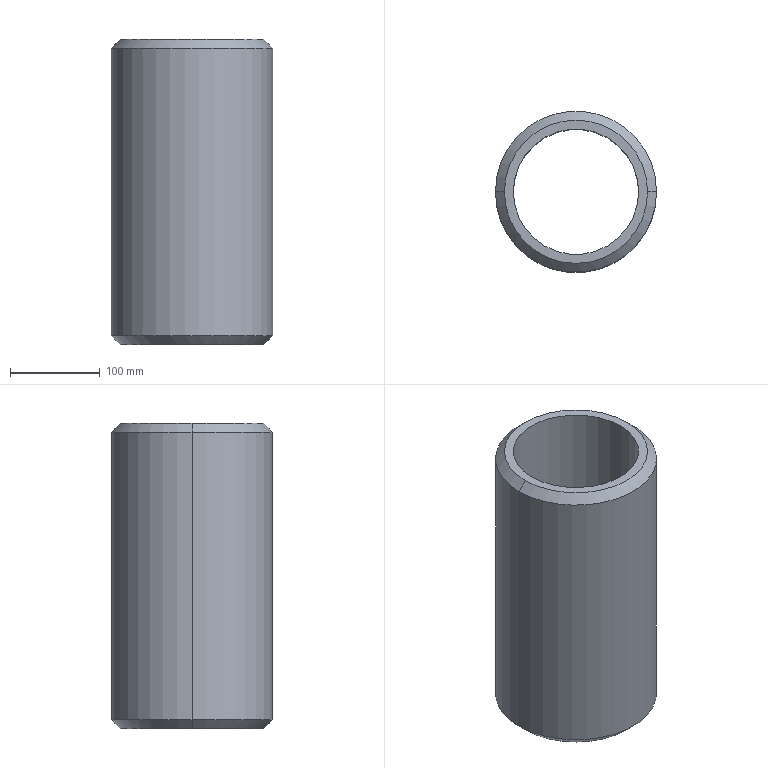Part | SolidWorks | features Chamfer 1, Extrusion 1 | 1 solid | 10 faces | box 180 x 180 x 341 mm | volume 3373652 mm3 | cone 4 | cylinder 4 | plane 2 | commonest cylinder face diameters 140 x2 180 x2
STEP:
#1=CARTESIAN_POINT('',(80.,0.,341.));
#2=VERTEX_POINT('',#1);
#3=CARTESIAN_POINT('',(-80.,0.,341.));
#4=VERTEX_POINT('',#3);
#5=CARTESIAN_POINT('',(0.,0.,341.));
#6=DIRECTION('',(0.,0.,1.));
#7=DIRECTION('',(1.,0.,0.));
#8=AXIS2_PLACEMENT_3D('',#5,#6,#7);
#9=CIRCLE('',#8,80.);
#10=EDGE_CURVE('',#2,#4,#9,.T.);
#11=ORIENTED_EDGE('',*,*,#10,.F.);
#12=CARTESIAN_POINT('',(90.,0.,331.));
#13=VERTEX_POINT('',#12);
#14=CARTESIAN_POINT('',(80.,0.,341.));
#15=DIRECTION('',(0.7071,0.,-0.7071));
#16=VECTOR('',#15,1000.);
#17=LINE('',#14,#16);
#18=EDGE_CURVE('',#2,#13,#17,.T.);
#19=ORIENTED_EDGE('',*,*,#18,.T.);
#20=CARTESIAN_POINT('',(-90.,0.,331.));
#21=VERTEX_POINT('',#20);
#22=CARTESIAN_POINT('',(0.,0.,331.));
#23=DIRECTION('',(0.,0.,-1.));
#24=DIRECTION('',(1.,0.,0.));
#25=AXIS2_PLACEMENT_3D('',#22,#23,#24);
#26=CIRCLE('',#25,90.);
#27=EDGE_CURVE('',#21,#13,#26,.T.);
#28=ORIENTED_EDGE('',*,*,#27,.F.);
#29=CARTESIAN_POINT('',(-80.,0.,341.));
#30=DIRECTION('',(-0.7071,0.,-0.7071));
#31=VECTOR('',#30,1000.);
#32=LINE('',#29,#31);
#33=EDGE_CURVE('',#4,#21,#32,.T.);
#34=ORIENTED_EDGE('',*,*,#33,.F.);
#35=EDGE_LOOP('',(#11,#19,#28,#34));
#36=FACE_OUTER_BOUND('',#35,.T.);
#37=CARTESIAN_POINT('',(0.,0.,341.));
#38=DIRECTION('',(0.,0.,-1.));
#39=DIRECTION('',(-1.,0.,0.));
#40=AXIS2_PLACEMENT_3D('',#37,#38,#39);
#41=CONICAL_SURFACE('',#40,80.,0.7854);
#42=ADVANCED_FACE('',(#36),#41,.T.);
#43=CARTESIAN_POINT('',(-80.,0.,0.));
#44=VERTEX_POINT('',#43);
#45=CARTESIAN_POINT('',(80.,0.,0.));
#46=VERTEX_POINT('',#45);
#47=CARTESIAN_POINT('',(0.,0.,0.));
#48=DIRECTION('',(0.,0.,-1.));
#49=DIRECTION('',(1.,0.,0.));
#50=AXIS2_PLACEMENT_3D('',#47,#48,#49);
#51=CIRCLE('',#50,80.);
#52=EDGE_CURVE('',#44,#46,#51,.T.);
#53=ORIENTED_EDGE('',*,*,#52,.F.);
#54=CARTESIAN_POINT('',(-90.,0.,10.));
#55=VERTEX_POINT('',#54);
#56=CARTESIAN_POINT('',(-90.,0.,10.));
#57=DIRECTION('',(-0.7071,0.,0.7071));
#58=VECTOR('',#57,1000.);
#59=LINE('',#56,#58);
#60=EDGE_CURVE('',#44,#55,#59,.T.);
#61=ORIENTED_EDGE('',*,*,#60,.T.);
#62=CARTESIAN_POINT('',(90.,0.,10.));
#63=VERTEX_POINT('',#62);
#64=CARTESIAN_POINT('',(0.,0.,10.));
#65=DIRECTION('',(0.,0.,1.));
#66=DIRECTION('',(1.,0.,0.));
#67=AXIS2_PLACEMENT_3D('',#64,#65,#66);
#68=CIRCLE('',#67,90.);
#69=EDGE_CURVE('',#63,#55,#68,.T.);
#70=ORIENTED_EDGE('',*,*,#69,.F.);
#71=CARTESIAN_POINT('',(90.,0.,10.));
#72=DIRECTION('',(0.7071,0.,0.7071));
#73=VECTOR('',#72,1000.);
#74=LINE('',#71,#73);
#75=EDGE_CURVE('',#46,#63,#74,.T.);
#76=ORIENTED_EDGE('',*,*,#75,.F.);
#77=EDGE_LOOP('',(#53,#61,#70,#76));
#78=FACE_OUTER_BOUND('',#77,.T.);
#79=CARTESIAN_POINT('',(0.,0.,10.));
#80=DIRECTION('',(0.,0.,1.));
#81=DIRECTION('',(1.,0.,0.));
#82=AXIS2_PLACEMENT_3D('',#79,#80,#81);
#83=CONICAL_SURFACE('',#82,90.,0.7854);
#84=ADVANCED_FACE('',(#78),#83,.T.);
#85=CARTESIAN_POINT('',(-70.,0.,341.));
#86=VERTEX_POINT('',#85);
#87=CARTESIAN_POINT('',(70.,0.,341.));
#88=VERTEX_POINT('',#87);
#89=CARTESIAN_POINT('',(0.,0.,341.));
#90=DIRECTION('',(0.,0.,1.));
#91=DIRECTION('',(1.,0.,0.));
#92=AXIS2_PLACEMENT_3D('',#89,#90,#91);
#93=CIRCLE('',#92,70.);
#94=EDGE_CURVE('',#86,#88,#93,.T.);
#95=ORIENTED_EDGE('',*,*,#94,.T.);
#96=CARTESIAN_POINT('',(70.,0.,0.));
#97=VERTEX_POINT('',#96);
#98=CARTESIAN_POINT('',(70.,0.,341.));
#99=DIRECTION('',(0.,0.,-1.));
#100=VECTOR('',#99,1000.);
#101=LINE('',#98,#100);
#102=EDGE_CURVE('',#88,#97,#101,.T.);
#103=ORIENTED_EDGE('',*,*,#102,.T.);
#104=CARTESIAN_POINT('',(-70.,0.,0.));
#105=VERTEX_POINT('',#104);
#106=CARTESIAN_POINT('',(0.,0.,0.));
#107=DIRECTION('',(0.,0.,1.));
#108=DIRECTION('',(1.,0.,0.));
#109=AXIS2_PLACEMENT_3D('',#106,#107,#108);
#110=CIRCLE('',#109,70.);
#111=EDGE_CURVE('',#105,#97,#110,.T.);
#112=ORIENTED_EDGE('',*,*,#111,.F.);
#113=CARTESIAN_POINT('',(-70.,0.,341.));
#114=DIRECTION('',(0.,0.,-1.));
#115=VECTOR('',#114,1000.);
#116=LINE('',#113,#115);
#117=EDGE_CURVE('',#86,#105,#116,.T.);
#118=ORIENTED_EDGE('',*,*,#117,.F.);
#119=EDGE_LOOP('',(#95,#103,#112,#118));
#120=FACE_OUTER_BOUND('',#119,.T.);
#121=CARTESIAN_POINT('',(0.,0.,341.));
#122=DIRECTION('',(0.,0.,-1.));
#123=DIRECTION('',(-1.,0.,0.));
#124=AXIS2_PLACEMENT_3D('',#121,#122,#123);
#125=CYLINDRICAL_SURFACE('',#124,70.);
#126=ADVANCED_FACE('',(#120),#125,.F.);
#127=ORIENTED_EDGE('',*,*,#27,.T.);
#128=CARTESIAN_POINT('',(90.,0.,341.));
#129=DIRECTION('',(0.,0.,-1.));
#130=VECTOR('',#129,1000.);
#131=LINE('',#128,#130);
#132=EDGE_CURVE('',#13,#63,#131,.T.);
#133=ORIENTED_EDGE('',*,*,#132,.T.);
#134=ORIENTED_EDGE('',*,*,#69,.T.);
#135=CARTESIAN_POINT('',(-90.,0.,341.));
#136=DIRECTION('',(0.,0.,-1.));
#137=VECTOR('',#136,1000.);
#138=LINE('',#135,#137);
#139=EDGE_CURVE('',#21,#55,#138,.T.);
#140=ORIENTED_EDGE('',*,*,#139,.F.);
#141=EDGE_LOOP('',(#127,#133,#134,#140));
#142=FACE_OUTER_BOUND('',#141,.T.);
#143=CARTESIAN_POINT('',(0.,0.,341.));
#144=DIRECTION('',(0.,0.,-1.));
#145=DIRECTION('',(-1.,0.,0.));
#146=AXIS2_PLACEMENT_3D('',#143,#144,#145);
#147=CYLINDRICAL_SURFACE('',#146,90.);
#148=ADVANCED_FACE('',(#142),#147,.T.);
#149=CARTESIAN_POINT('',(0.,0.,341.));
#150=DIRECTION('',(0.,0.,1.));
#151=DIRECTION('',(1.,0.,0.));
#152=AXIS2_PLACEMENT_3D('',#149,#150,#151);
#153=CIRCLE('',#152,80.);
#154=EDGE_CURVE('',#4,#2,#153,.T.);
#155=ORIENTED_EDGE('',*,*,#154,.T.);
#156=ORIENTED_EDGE('',*,*,#10,.T.);
#157=EDGE_LOOP('',(#155,#156));
#158=FACE_OUTER_BOUND('',#157,.T.);
#159=ORIENTED_EDGE('',*,*,#94,.F.);
#160=CARTESIAN_POINT('',(0.,0.,341.));
#161=DIRECTION('',(0.,0.,1.));
#162=DIRECTION('',(1.,0.,0.));
#163=AXIS2_PLACEMENT_3D('',#160,#161,#162);
#164=CIRCLE('',#163,70.);
#165=EDGE_CURVE('',#88,#86,#164,.T.);
#166=ORIENTED_EDGE('',*,*,#165,.F.);
#167=EDGE_LOOP('',(#159,#166));
#168=FACE_BOUND('',#167,.T.);
#169=CARTESIAN_POINT('',(0.,0.,341.));
#170=DIRECTION('',(0.,0.,1.));
#171=DIRECTION('',(1.,0.,0.));
#172=AXIS2_PLACEMENT_3D('',#169,#170,#171);
#173=PLANE('',#172);
#174=ADVANCED_FACE('',(#158,#168),#173,.T.);
#175=CARTESIAN_POINT('',(0.,0.,0.));
#176=DIRECTION('',(0.,0.,-1.));
#177=DIRECTION('',(1.,0.,0.));
#178=AXIS2_PLACEMENT_3D('',#175,#176,#177);
#179=CIRCLE('',#178,80.);
#180=EDGE_CURVE('',#46,#44,#179,.T.);
#181=ORIENTED_EDGE('',*,*,#180,.T.);
#182=ORIENTED_EDGE('',*,*,#52,.T.);
#183=EDGE_LOOP('',(#181,#182));
#184=FACE_OUTER_BOUND('',#183,.T.);
#185=ORIENTED_EDGE('',*,*,#111,.T.);
#186=CARTESIAN_POINT('',(0.,0.,0.));
#187=DIRECTION('',(0.,0.,1.));
#188=DIRECTION('',(1.,0.,0.));
#189=AXIS2_PLACEMENT_3D('',#186,#187,#188);
#190=CIRCLE('',#189,70.);
#191=EDGE_CURVE('',#97,#105,#190,.T.);
#192=ORIENTED_EDGE('',*,*,#191,.T.);
#193=EDGE_LOOP('',(#185,#192));
#194=FACE_BOUND('',#193,.T.);
#195=CARTESIAN_POINT('',(0.,0.,0.));
#196=DIRECTION('',(0.,0.,1.));
#197=DIRECTION('',(1.,0.,0.));
#198=AXIS2_PLACEMENT_3D('',#195,#196,#197);
#199=PLANE('',#198);
#200=ADVANCED_FACE('',(#184,#194),#199,.F.);
#201=ORIENTED_EDGE('',*,*,#132,.F.);
#202=CARTESIAN_POINT('',(0.,0.,331.));
#203=DIRECTION('',(0.,0.,-1.));
#204=DIRECTION('',(1.,0.,0.));
#205=AXIS2_PLACEMENT_3D('',#202,#203,#204);
#206=CIRCLE('',#205,90.);
#207=EDGE_CURVE('',#13,#21,#206,.T.);
#208=ORIENTED_EDGE('',*,*,#207,.T.);
#209=ORIENTED_EDGE('',*,*,#139,.T.);
#210=CARTESIAN_POINT('',(0.,0.,10.));
#211=DIRECTION('',(0.,0.,1.));
#212=DIRECTION('',(1.,0.,0.));
#213=AXIS2_PLACEMENT_3D('',#210,#211,#212);
#214=CIRCLE('',#213,90.);
#215=EDGE_CURVE('',#55,#63,#214,.T.);
#216=ORIENTED_EDGE('',*,*,#215,.T.);
#217=EDGE_LOOP('',(#201,#208,#209,#216));
#218=FACE_OUTER_BOUND('',#217,.T.);
#219=CARTESIAN_POINT('',(0.,0.,341.));
#220=DIRECTION('',(0.,0.,-1.));
#221=DIRECTION('',(-1.,0.,0.));
#222=AXIS2_PLACEMENT_3D('',#219,#220,#221);
#223=CYLINDRICAL_SURFACE('',#222,90.);
#224=ADVANCED_FACE('',(#218),#223,.T.);
#225=ORIENTED_EDGE('',*,*,#102,.F.);
#226=ORIENTED_EDGE('',*,*,#165,.T.);
#227=ORIENTED_EDGE('',*,*,#117,.T.);
#228=ORIENTED_EDGE('',*,*,#191,.F.);
#229=EDGE_LOOP('',(#225,#226,#227,#228));
#230=FACE_OUTER_BOUND('',#229,.T.);
#231=CARTESIAN_POINT('',(0.,0.,341.));
#232=DIRECTION('',(0.,0.,-1.));
#233=DIRECTION('',(-1.,0.,0.));
#234=AXIS2_PLACEMENT_3D('',#231,#232,#233);
#235=CYLINDRICAL_SURFACE('',#234,70.);
#236=ADVANCED_FACE('',(#230),#235,.F.);
#237=ORIENTED_EDGE('',*,*,#60,.F.);
#238=ORIENTED_EDGE('',*,*,#180,.F.);
#239=ORIENTED_EDGE('',*,*,#75,.T.);
#240=ORIENTED_EDGE('',*,*,#215,.F.);
#241=EDGE_LOOP('',(#237,#238,#239,#240));
#242=FACE_OUTER_BOUND('',#241,.T.);
#243=CARTESIAN_POINT('',(0.,0.,10.));
#244=DIRECTION('',(0.,0.,1.));
#245=DIRECTION('',(1.,0.,0.));
#246=AXIS2_PLACEMENT_3D('',#243,#244,#245);
#247=CONICAL_SURFACE('',#246,90.,0.7854);
#248=ADVANCED_FACE('',(#242),#247,.T.);
#249=ORIENTED_EDGE('',*,*,#18,.F.);
#250=ORIENTED_EDGE('',*,*,#154,.F.);
#251=ORIENTED_EDGE('',*,*,#33,.T.);
#252=ORIENTED_EDGE('',*,*,#207,.F.);
#253=EDGE_LOOP('',(#249,#250,#251,#252));
#254=FACE_OUTER_BOUND('',#253,.T.);
#255=CARTESIAN_POINT('',(0.,0.,341.));
#256=DIRECTION('',(0.,0.,-1.));
#257=DIRECTION('',(-1.,0.,0.));
#258=AXIS2_PLACEMENT_3D('',#255,#256,#257);
#259=CONICAL_SURFACE('',#258,80.,0.7854);
#260=ADVANCED_FACE('',(#254),#259,.T.);
#261=CLOSED_SHELL('',(#42,#84,#126,#148,#174,#200,#224,#236,#248,#260));
#262=MANIFOLD_SOLID_BREP('',#261);
#263=CARTESIAN_POINT('',(0.,0.,0.));
#264=DIRECTION('',(0.,0.,1.));
#265=DIRECTION('',(1.,0.,0.));
#266=AXIS2_PLACEMENT_3D('',#263,#264,#265);
#267=(LENGTH_UNIT()NAMED_UNIT(*)SI_UNIT(.MILLI.,.METRE.));
#268=UNCERTAINTY_MEASURE_WITH_UNIT(LENGTH_MEASURE(0.00001),#267,'','');
#269=(NAMED_UNIT(*)PLANE_ANGLE_UNIT()SI_UNIT($,.RADIAN.));
#270=(NAMED_UNIT(*)SI_UNIT($,.STERADIAN.)SOLID_ANGLE_UNIT());
#271=(GEOMETRIC_REPRESENTATION_CONTEXT(3)GLOBAL_UNCERTAINTY_ASSIGNED_CONTEXT((#268))GLOBAL_UNIT_ASSIGNED_CONTEXT((#267,#269,#270))REPRESENTATION_CONTEXT('',''));
#272=ADVANCED_BREP_SHAPE_REPRESENTATION('',(#262,#266),#271);